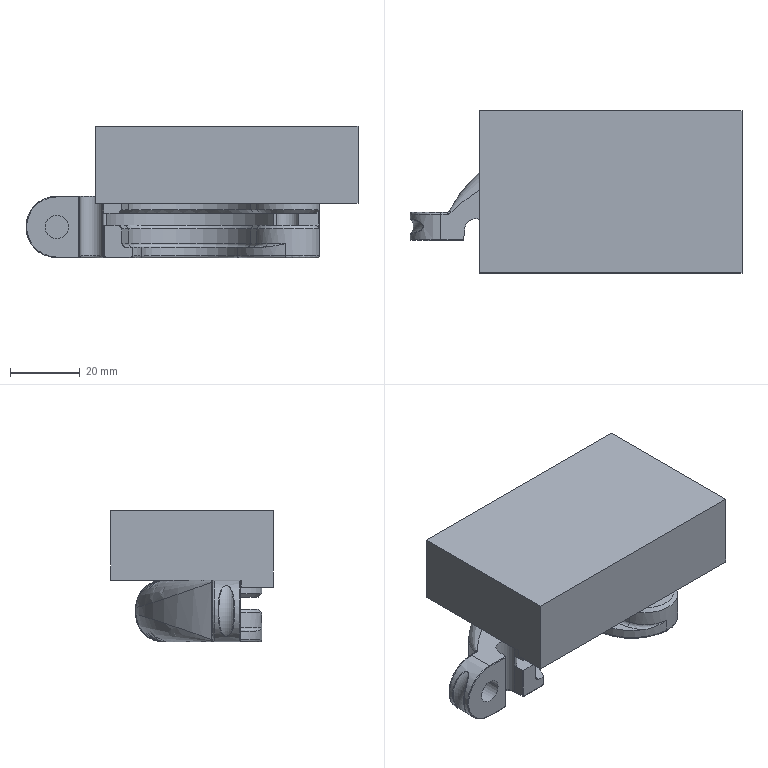NC program | NX | posted with a generic post | part box 94.951 x 46.35 x 37.6 mm
Lines 1 to 1739 of 15115, first 1433 of 1715 lines:
N10 G17 G21 G94 G90
(FACE_MILLING , TOOL : D63面刀)
N12 T01 M6
N14 G54
N16 G17 G0 G90 X104.291 Y-3.752 S4500 M3
N18 G43 Z20. H1
N20 Z3.
N22 G94 G1 Z0. F900.
N24 X72.643
N26 X-64.675 F1500.
N28 X-96.175
N30 Z3.
N32 G0 Z20.
N34 M5
(ADAPTIVE_MILLING , TOOL : D8开粗)
N36 T19 M6
N38 G54
N40 G17 G0 G90 X-51.02 Y-4.719 S6500 M3
N42 G43 Z20. H19
N44 Z-17.
N46 G94 G1 Z-20. F2100.
N48 X-49.643 Y-4.596 F3500.
N50 G3 X-49.006 Y-4.179 R0.813
N52 X-48.262 Y-1.372 R7.176
N54 X-47.978 Y7.018 R88.809
N56 G1 X-47.951 Y18.882
N58 G2 X-45.584 Y22.239 R4.73
N60 X-40.599 Y23.745 R12.005
N62 X-30.984 Y24.063 R95.907
N64 G1 X-26.234 Y24.068
N66 X42.508 Y24.067
N68 G2 X45.905 Y21.99 R4.502
N70 X47.594 Y17.053 R10.976
N72 X47.954 Y8.941 R70.776
N74 G1 X47.967 Y2.441
N76 X47.966 Y-18.643
N78 G2 X45.892 Y-22.039 R4.468
N80 X41.089 Y-23.684 R10.837
N82 X32.103 Y-24.059 R75.64
N84 G1 X25.978 Y-24.068
N86 X-42.494 Y-24.067
N88 G2 X-45.912 Y-22.034 R4.428
N90 X-47.595 Y-17.116 R10.874
N92 X-47.953 Y-9.129 R69.614
N94 X-47.555 Y-3.593 R27.936
N96 G3 X-46.984 Y8.023 R94.067
N98 G2 X-46.932 Y16.506 R267.577
N100 X-43.634 Y21.111 R6.219
N102 X-37.776 Y22.742 R14.951
N104 X-27.66 Y23.063 R109.609
N106 G1 X-23.535 Y23.067
N108 X39.857 Y23.066
N110 G2 X44.856 Y19.967 R6.087
N112 X46.593 Y14.273 R13.924
N114 X46.959 Y4.66 R91.618
N116 G1 X46.967 Y-2.215
N118 X46.944 Y-16.393
N120 G2 X43.82 Y-21.002 R6.125
N122 X38.236 Y-22.689 R13.96
N124 X28.476 Y-23.057 R91.812
N126 G1 X23.476 Y-23.067
N128 X-39.918 Y-23.065
N130 G2 X-44.82 Y-20.054 R6.012
N132 X-46.553 Y-14.619 R13.397
N134 X-46.497 Y-3.336 R45.895
N136 G3 X-45.978 Y10.393 R148.883
N138 G2 X-45.891 Y14.755 R46.886
N140 X-42.059 Y20.004 R7.121
N142 X-35.83 Y21.713 R16.455
N144 X-25.965 Y22.059 R104.665
N146 G1 X-19.09 Y22.067
N148 X0.976
N150 X2.332 Y22.205
N152 G2 X8.926 Y22.127 R73.557
N154 G1 X15.608 Y22.068
N156 X37.558 Y22.065
N158 G2 X43.868 Y18.207 R7.099
N160 X45.592 Y12.1 R16.115
N162 X45.96 Y1.611 R105.759
N164 G1 X45.967 Y-6.863
N166 X46.121 Y-7.731
N168 G2 X45.929 Y-14.694 R100.465
N170 X42.014 Y-20.037 R7.181
N172 X36.996 Y-21.568 R15.133
N174 G1 X36.466 Y-21.769
N176 X34.201 Y-22.204
N178 G2 X28.896 Y-22.118 R65.764
N180 G1 X22.206 Y-22.068
N182 X-37.544 Y-22.067
N184 G2 X-43.799 Y-18.344 R7.037
N186 X-45.264 Y-14.372 R14.785
N188 X-46.031 Y-12.836 R5.048
N190 X-46.028 Y-8.948 R12.446
N192 G3 X-45.885 Y-7.084 R20.16
N194 G2 X-46.174 Y-4.608 R6.372
N196 X-45.719 Y-2.074 R11.118
N198 G3 X-45.051 Y6.078 R50.118
N200 G2 X-44.918 Y12.773 R198.768
N202 X-40.696 Y18.891 R7.78
N204 X-34.228 Y20.679 R17.366
N206 X-23.115 Y21.061 R112.747
N208 G1 X-18.99 Y21.067
N210 X-5.419 Y21.068
N212 X-1.618 Y21.803
N214 X2.332 Y22.205
N216 X6.303 Y22.25
N218 X10.261 Y21.94
N220 G3 X19.395 Y21.101 R42.809
N222 G1 X35.932 Y21.055
N224 G2 X42.861 Y16.652 R7.812
N226 X44.595 Y10.17 R17.88
N228 X44.96 Y-0.694 R114.167
N230 G1 X44.989 Y-3.46
N232 X45.717 Y-5.46
N234 X45.98 Y-6.937
N236 G3 X47.568 Y-6.813 R0.8
N238 G1 X47.661 Y-5.251 Z-19.9
N240 X47.74 Y-3.888
N242 X47.702 Y-0.81
N244 X47.617 Y2.267
N246 X47.499 Y4.315
N248 X47.338 Y6.36
N250 X47.052 Y9.524
N252 X46.747 Y12.687
N254 G3 X45.741 Y16.134 R13.079
N256 X44.088 Y19.29 R24.994
N258 X37.545 Y23.22 R8.856
N260 X33.163 Y23.495 R58.704
N262 G1 X15.727 Y23.898
N264 X15.524 Y23.849
N266 X14.073 Y23.289
N268 X13.077 Y22.895 Z-19.969
N270 G3 X12.75 Y22.537 Z-20. R0.846
N272 X13.342 Y21.413 R0.8
N274 G2 X16.779 Y20.595 R32.188
N276 G3 X23.653 Y20.109 R41.473
N278 G1 X34.557 Y20.036
N280 G2 X41.838 Y15.239 R8.359
N282 X43.576 Y8.62 R18.862
N284 X43.964 Y-1.334 R112.841
N286 G1 X44.021 Y-1.556
N288 G2 X45.014 Y-3.527 R30.259
N290 G3 X46.304 Y-3.845 R0.8
N292 X46.574 Y-3.166 Z-19.952 R0.899
N294 G1 X46.635 Y-2.357 Z-19.9
N296 X46.774 Y-0.478
N298 X46.776 Y1.281
N300 X46.73 Y3.039
N302 X46.635 Y4.206
N304 X46.497 Y5.37
N306 X45.704 Y10.852
N308 G3 X44.528 Y15.045 R20.143
N310 X43.203 Y17.473 R13.919
N312 G1 X42.516 Y18.481
N314 X41.794 Y19.464
N316 G3 X41.087 Y20.126 R3.656
N318 X36.954 Y22.042 R11.259
N320 G1 X36.341 Y22.149
N322 X35.722 Y22.22
N324 X32.067 Y22.476
N326 X28.41 Y22.683
N328 X19.055 Y23.131
N330 X18.882 Y23.116
N332 X18.714 Y23.072
N334 X17.29 Y22.49
N336 X16.816 Y22.298 Z-19.933
N338 X16.349 Y22.093 Z-19.965
N340 G3 X16.016 Y21.677 Z-20. R0.837
N342 X16.565 Y20.641 R0.8
N344 G2 X19.636 Y19.719 R46.577
N346 G3 X25.689 Y19.144 R31.586
N348 G2 X33.243 Y19.021 R667.849
N350 X40.794 Y13.949 R8.781
N352 X42.57 Y7.089 R19.793
N354 X42.94 Y0.558 R126.133
N356 G3 X44.028 Y-1.57 R111.415
N358 X45.191 Y-1.858 R0.8
N360 X45.547 Y-1.135 Z-19.947 R0.881
N362 G1 X45.621 Y-0.413 Z-19.9
N364 X45.796 Y1.382
N366 X45.252 Y5.256
N368 X44.683 Y9.127
N370 G3 X43.427 Y13.856 R27.88
N372 G1 X42.817 Y15.509
N374 G3 X41.412 Y17.59 R6.625
N376 X38.104 Y20.149 R16.811
N378 X35.162 Y21.088 R8.045
N380 G1 X32.008 Y21.444
N382 X28.848 Y21.745
N384 X21.628 Y22.348
N386 X21.431 Y22.337
N388 X21.24 Y22.283
N390 X19.885 Y21.688
N392 X18.991 Y21.287 Z-19.963
N394 G3 X18.647 Y20.83 Z-20. R0.83
N396 X19.139 Y19.858 R0.801
N398 X22.763 Y18.649 R25.814
N400 X29.299 Y18.13 R40.933
N402 G2 X34.012 Y17.673 R18.904
N404 X39.845 Y12.527 R9.247
N406 X41.589 Y5.394 R21.313
N408 G1 X41.851 Y2.231
N410 G3 X43.044 Y0.313 R15.776
N412 X44.116 Y0.055 R0.801
N414 X44.528 Y0.799 Z-19.943 R0.875
N416 G1 X44.61 Y1.469 Z-19.9
N418 X44.726 Y2.352
N420 X44.818 Y3.237
N422 G3 X42.965 Y11.077 R64.156
N424 X41.261 Y14.968 R19.576
N426 G1 X40.36 Y16.513
N428 G3 X38.875 Y17.974 R5.483
N430 X33.742 Y20.116 R13.869
N432 G1 X32.664 Y20.317
N434 X31.579 Y20.481
N436 X23.982 Y21.446
N438 X23.82 Y21.424
N440 X23.663 Y21.376
N442 X22.341 Y20.784
N444 X21.449 Y20.376 Z-19.963
N446 G3 X21.109 Y19.918 Z-20. R0.83
N448 X21.602 Y18.95 R0.801
N450 G1 X23.779 Y18.005
N452 G3 X28.447 Y17.268 R19.998
N454 G2 X33.008 Y16.627 R19.382
N456 X38.887 Y11.172 R9.701
N458 X40.548 Y4.469 R22.433
N460 G3 X40.836 Y3.73 R1.258
N462 G1 X41.921 Y2.05
N464 G3 X43.335 Y2.185 R0.8
N466 X43.335 Y2.857 Z-19.956 R1.091
N468 G1 X43.162 Y3.72 Z-19.9
N470 X42.836 Y5.372
N472 X42.831 Y5.98
N474 X42.785 Y6.587
N476 G3 X41.688 Y10.669 R25.729
N478 X40.431 Y13.306 R16.27
N480 G1 X39.455 Y14.928
N482 G3 X37.035 Y17.302 R8.254
N484 X33.086 Y19.162 R13.784
N486 X31.176 Y19.51 R11.526
N488 G1 X26.234 Y19.969
N490 X24.471 Y19.81
N492 X23.408 Y19.703 Z-19.968
N494 G3 X22.994 Y19.445 Z-20. R0.845
N496 X23.259 Y18.205 R0.8
N498 X26.334 Y16.884 R18.397
N500 X30.452 Y16.102 R99.604
N502 G2 X37.924 Y9.88 R10.25
N504 X39.185 Y5.864 R27.369
N506 G1 X40.782 Y3.799
N508 G3 X42.064 Y3.832 R0.8
N510 X42.172 Y4.584 Z-19.95 R0.9
N512 G1 X42.039 Y5.352 Z-19.9
N514 X41.728 Y7.106
N516 X40.782 Y9.234
N518 X39.816 Y11.353
N520 G3 X36.767 Y15.518 R13.967
N522 X33.532 Y17.631 R12.909
N524 X31.698 Y18.233 R10.561
N526 G1 X28.338 Y18.996
N528 X28.08 Y19.012
N530 X26.479 Y18.849
N532 X25.428 Y18.731 Z-19.968
N534 G3 X25.011 Y18.46 Z-20. R0.843
N536 X25.289 Y17.236 R0.8
N538 G1 X27.065 Y16.272
N540 X30.763 Y14.957
N542 G2 X37.032 Y8.501 R11.31
N544 G1 X37.242 Y8.072
N546 G2 X39.25 Y5.75 R19.09
N548 G3 X40.548 Y5.805 R0.8
N550 X40.638 Y6.536 Z-19.951 R0.896
N552 G1 X40.488 Y7.327 Z-19.9
N554 X40.39 Y7.864
N556 X40.274 Y8.398
N558 X40.179 Y8.574
N560 X40.047 Y8.725
N562 X29.323 Y18.01
N564 G3 X28.686 Y18.197 R0.808
N566 G1 X27.817 Y18.073
N568 X27.316 Y18.003 Z-19.932
N570 X26.817 Y17.918 Z-19.965
N572 G3 X26.39 Y17.586 Z-20. R0.836
N574 X26.656 Y16.47 R0.8
N576 G2 X31.937 Y13.115 R52.707
N578 X33.4 Y11.755 R22.501
N580 X37.246 Y8.068 R34.365
N582 G3 X38.5 Y9.053 R0.801
N584 G1 X37.718 Y10.408 Z-19.9
N586 X37.331 Y11.058
N588 X37.246 Y11.149
N590 X32.159 Y15.761
N592 X31.989 Y15.876
N594 X31.797 Y15.949
N596 X30.891 Y16.153
N598 X29.712 Y16.409 Z-19.977
N600 X29.534 Y16.398 Z-19.989
N602 X29.361 Y16.355 Z-20.
N604 G3 X29.184 Y14.964 R0.8
N606 G1 X32.473 Y12.57
N608 X33.412 Y11.745
N610 G3 X34.209 Y11.592 R0.803
N612 G1 X34.462 Y11.739 Z-19.981
N614 X34.685 Y11.928 Z-19.963
N616 X35.434 Y12.558 Z-19.9
N618 X35.651 Y12.742
N620 X35.894 Y12.893
N622 G2 X36.812 Y12.656 R0.801
N624 G1 X40.201 Y8.483
N626 G2 X43.948 Y3.357 R76.172
N628 X45.937 Y-0.004 R46.197
N630 G1 X47.032 Y-2.073
N632 G2 X48.199 Y-5.501 R14.427
N634 G1 X48.618 Y-7.549
N636 G2 X48.259 Y-8.387 R0.802
N638 G1 X48.104 Y-8.484
N640 X46.778 Y-9.316 Z-20.
N642 X46.521 Y-9.475
N644 G3 X46.128 Y-10.038 R0.908
N646 G2 X45.654 Y-12.547 R19.534
N648 X43.824 Y-16.49 R11.526
N650 G1 X42.358 Y-18.271
N652 X40.607 Y-19.772
N654 X38.623 Y-20.95
N656 X36.987 Y-21.571
N658 G3 X36.606 Y-22.764 R0.8
N660 X37.292 Y-23.133 Z-19.948 R0.892
N662 G1 X38.039 Y-23.255 Z-19.9
N664 X38.795 Y-23.384
N666 X39.555 Y-23.491
N668 G3 X40.036 Y-23.331 R0.825
N670 G1 X42.47 Y-21.491
N672 G3 X45.378 Y-18.415 R16.117
N674 G1 X47.414 Y-15.596
N676 G3 X47.556 Y-15.005 R0.812
N678 G1 X47.348 Y-13.658
N680 X47.172 Y-12.579 Z-19.97
N682 G3 X46.912 Y-12.195 Z-20. R0.852
N684 X45.654 Y-12.547 R0.8
N686 G1 X44.962 Y-14.484
N688 X43.824 Y-16.49
N690 X42.358 Y-18.271
N692 X40.607 Y-19.772
N694 X38.623 Y-20.95
N696 X36.466 Y-21.769
N698 X34.201 Y-22.204
N700 X31.895 Y-22.242
N702 X29.155 Y-21.851
N704 G3 X24.557 Y-21.196 R17.279
N706 X14.706 Y-21.068 R300.396
N708 G1 X-35.494 Y-21.066
N710 G2 X-42.791 Y-16.805 R7.835
N712 G3 X-43.475 Y-15.763 R3.342
N714 G2 X-45.347 Y-14.231 R4.167
N716 G3 X-46.728 Y-15.009 R0.8
N718 G1 X-46.029 Y-16.408 Z-19.9
N720 X-45.347 Y-17.751
N722 X-44.862 Y-18.482
N724 X-44.341 Y-19.189
N726 X-43.95 Y-19.622
N728 X-43.532 Y-20.029
N730 X-42.119 Y-21.273
N732 G3 X-36.704 Y-23.29 R8.961
N734 G1 X-34.755 Y-23.394
N736 X-32.804 Y-23.447
N738 X26.052 Y-24.123
N740 X26.258 Y-24.069
N742 X27.697 Y-23.481
N744 X28.169 Y-23.29 Z-19.933
N746 X28.634 Y-23.085 Z-19.965
N748 G3 X28.967 Y-22.664 Z-20. R0.836
N750 X28.435 Y-21.64 R0.8
N752 X25.125 Y-20.647 R152.961
N754 X18.279 Y-20.117 R39.289
N756 G1 X10.831 Y-20.068
N758 X-33.619 Y-20.066
N760 G2 X-38.961 Y-18.63 R9.039
N762 X-41.575 Y-16.272 R25.088
N764 G1 X-41.929 Y-16.103
N766 G2 X-43.601 Y-15.689 R4.008
N768 G3 X-44.704 Y-16.364 R0.8
N770 X-44.429 Y-17.052 Z-19.951 R0.894
N772 G1 X-43.917 Y-17.666 Z-19.9
N774 X-42.781 Y-19.019
N776 X-41.518 Y-19.872
N778 X-40.243 Y-20.707
N780 G3 X-35.676 Y-22.237 R11.641
N782 X-32.268 Y-22.421 R35.503
N784 G1 X23.411 Y-22.775
N786 X25.17 Y-22.624
N788 X26.241 Y-22.522 Z-19.969
N790 G3 X26.653 Y-22.274 Z-20. R0.847
N792 X26.386 Y-21.018 R0.8
N794 X23.294 Y-19.769 R16.508
N796 X16.751 Y-19.147 R34.278
N798 X6.832 Y-19.068 R613.153
N800 G1 X-31.618 Y-19.067
N802 G2 X-36.626 Y-18.205 R11.616
N804 X-39.691 Y-16.358 R25.242
N806 G3 X-40.254 Y-16.125 R2.099
N808 G2 X-42.01 Y-16.093 R37.287
N810 G3 X-42.892 Y-17.069 R0.8
N812 X-42.421 Y-17.638 Z-19.951 R0.895
N814 G1 X-41.746 Y-18.071 Z-19.9
N816 X-41.248 Y-18.393
N818 X-40.74 Y-18.7
N820 X-40.47 Y-18.76
N822 X21.829 Y-21.672
N824 X23.097 Y-21.665
N826 X23.678 Y-21.663 Z-19.937
N828 X24.259 Y-21.646 Z-19.974
N830 X24.449 Y-21.584 Z-19.987
N832 X24.622 Y-21.482 Z-20.
N834 G3 X24.455 Y-20.131 R0.8
N836 G2 X23.154 Y-19.4 R10.946
N838 G3 X18.77 Y-18.391 R13.255
N840 X8.823 Y-18.077 R119.783
N842 G1 X-29.244 Y-18.069
N844 G2 X-34.207 Y-17.621 R18.247
N846 X-37.772 Y-16.167 R22.758
N848 G1 X-37.959 Y-16.125
N850 X-40.334
N852 G3 X-40.379 Y-17.884 R0.88
N854 G1 X-38.122 Y-17.999
N856 X-36.559 Y-18.08 Z-19.9
N858 X22.182 Y-21.092
N860 X22.962 Y-21.122 Z-19.95
N862 G3 X23.611 Y-20.73 Z-20. R0.895
N864 X23.355 Y-19.507 R0.88
N866 X20.583 Y-18.043 R9.835
N868 X14.436 Y-17.225 R26.833
N870 X2.332 Y-17.069 R314.868
N872 G1 X-34.442 Y-17.047
N874 X-35.922 Y-16.185
N876 X-36.168 Y-16.125
N878 X-38.043
N880 G3 X-38.078 Y-17.884 R0.88
N882 G1 X-34.699 Y-18.018
N884 X-33.136 Y-18.08 Z-19.9
N886 X20.83 Y-20.217
N888 X21.608 Y-20.238 Z-19.95
N890 G3 X22.254 Y-19.836 Z-20. R0.895
N892 X21.991 Y-18.624 R0.88
N894 G2 X20.98 Y-17.855 R23.145
N896 G3 X16.757 Y-16.576 R11.091
N898 X7.181 Y-16.094 R80.358
N900 G1 X1.706 Y-16.069
N902 X-11.094
N904 X-11.564 Y-16.125
N906 G2 X-26.403 Y-16.073 R924.171
N908 G1 X-26.834 Y-16.125
N910 X-36.209
N912 G3 X-36.505 Y-17.668 R0.8
N914 G1 X-34.995 Y-18.075 Z-19.9
N916 X-34.135 Y-18.296
N918 X-21.696 Y-18.303
N920 X-21.484 Y-18.274
N922 X-20.52 Y-18.009
N924 X-19.257 Y-17.65 Z-19.984
N926 X-19.048 Y-17.513 Z-20.
N928 G3 X-19.518 Y-16.125 R0.8
N930 G2 X-21.575 Y-15.691 R5.213
N932 G3 X-24.205 Y-15.318 R11.691
N934 X-24.793 Y-15.623 R1.742
N936 G2 X-26.403 Y-16.073 R4.48
N938 G3 X-26.344 Y-17.825 R0.88
N940 G1 X-24.785 Y-17.705 Z-19.9
N942 X-22.31 Y-17.501
N944 X-21.876 Y-17.47 Z-19.928
N946 X-21.446 Y-17.407 Z-19.956
N948 G3 X-20.924 Y-16.978 Z-20. R0.886
N950 X-21.408 Y-15.739 R0.88
N952 G2 X-22.367 Y-15.202 R9.846
N954 G3 X-23.766 Y-14.952 R1.975
N956 G1 X-24.539 Y-15.449
N958 G3 X-24.812 Y-16.596 R0.881
N960 X-23.863 Y-17.048 Z-19.929 R0.934
N962 G1 X-23.418 Y-17.034 Z-19.9
N964 X-23.106 Y-17.023
N966 X-22.339 Y-16.988 Z-19.949
N968 G3 X-21.72 Y-16.531 Z-20. R0.895
N970 X-22.007 Y-15.393 R0.881
N972 X-23.018 Y-14.748 R6.658
N974 X-24.024 Y-15.095 R1.114
N976 X-23.127 Y-16.604 R0.88
N978 G1 X-22.644 Y-16.346
N980 G3 X-22.5 Y-15.06 R0.88
N982 X-23.87 Y-14.967 R0.874
N984 X-24.064 Y-15.485 R0.819
N986 G1 X-24.065 Y-15.871
N988 X-24.069 Y-17.436 Z-19.9
N990 G2 X-24.782 Y-18.367 R0.834
N992 G1 X-26.53 Y-18.563
N994 X-28.282 Y-18.714
N996 X-29.453 Y-18.753
N998 X-30.624 Y-18.751
N1000 X-42.659 Y-18.456
N1002 G2 X-47.681 Y-15.035 R5.577
N1004 G1 X-48.65 Y-12.703
N1006 G2 X-48.158 Y-11.623 R0.832
N1008 G1 X-46.768 Y-10.903 Z-20.
N1010 G3 X-46.236 Y-10.454 R1.036
N1012 X-45.987 Y-9.024 R10.911
N1014 X-45.577 Y-7.92 R3.207
N1016 X-45.945 Y-6.889 R3.239
N1018 G2 X-46.174 Y-4.608 R6.402
N1020 G1 X-46.048 Y-3.343
N1022 G2 X-45.129 Y-1.225 R23.425
N1024 G3 X-44.22 Y4.097 R19.795
N1026 X-43.954 Y10.936 R538.277
N1028 G2 X-39.17 Y17.933 R8.368
N1030 X-32.558 Y19.675 R18.833
N1032 X-21.819 Y20.058 R112.509
N1034 G1 X-8.882 Y20.078
N1036 X-5.394 Y21.073
N1038 G3 X-5.17 Y22.565 R0.8
N1040 X-5.726 Y22.671 Z-19.964 R1.279
N1042 G1 X-6.718 Y22.73 Z-19.9
N1044 X-8.443 Y22.833
N1046 X-22.622
N1048 G3 X-31.385 Y22.252 R66.484
N1050 G1 X-33.242 Y22.008
N1052 X-35.093 Y21.723
N1054 G3 X-39.193 Y20.556 R21.136
N1056 X-42.298 Y18.863 R17.245
N1058 X-45.501 Y14.532 R9.105
N1060 X-46.164 Y11.699 R12.855
N1062 G1 X-46.42 Y9.764
N1064 X-46.642 Y7.824
N1066 X-47.352 Y0.799
N1068 X-47.134 Y-0.924
N1070 X-46.999 Y-1.896 Z-19.963
N1072 G3 X-46.66 Y-2.354 Z-20. R0.83
N1074 X-45.588 Y-2.158 R0.801
N1076 X-43.64 Y2.224 R8.412
N1078 X-43.042 Y9.021 R55.93
N1080 G2 X-37.661 Y17.002 R9.017
N1082 X-30.774 Y18.695 R20.684
N1084 X-18.659 Y19.062 R136.64
N1086 G1 X-11.643 Y19.075
N1088 G2 X-8.851 Y20.087 R56.002
N1090 G3 X-8.598 Y21.499 R0.8
N1092 X-9.24 Y21.669 Z-19.957 R1.099
N1094 G1 X-10.126 Y21.729 Z-19.9
N1096 X-11.9 Y21.847
N1098 X-20.701
N1100 G3 X-30.431 Y21.156 R68.93
N1102 G1 X-33.977 Y20.638
N1104 G3 X-38.469 Y19.26 R20.042
N1106 X-40.74 Y17.861 R12.305
N1108 X-43.034 Y15.917 R26.005
N1110 X-44.586 Y13.191 R6.411
N1112 X-45.647 Y8.034 R54.798
N1114 G1 X-46.597 Y1.816
N1116 X-46.58 Y1.626
N1118 X-46.282 Y0.2
N1120 X-46.062 Y-0.799 Z-19.965
N1122 G3 X-45.715 Y-1.201 Z-20. R0.837
N1124 X-44.828 Y-1.138 R0.802
N1126 X-43.333 Y1.006 R4.387
N1128 X-42.288 Y6.422 R20.895
N1130 G2 X-41.317 Y11.173 R14.886
N1132 X-35.891 Y16.21 R9.905
N1134 X-28.46 Y17.768 R24.307
N1136 X-16.216 Y18.06 R169.565
N1138 G3 X-13.9 Y18.097 R32.081
N1140 G2 X-11.401 Y19.144 R25.984
N1142 G3 X-11.116 Y20.446 R0.8
N1144 X-11.78 Y20.699 Z-19.953 R0.909
N1146 G1 X-12.612 Y20.764 Z-19.9
N1148 X-14.45 Y20.904
N1150 X-20.106 Y20.892
N1152 G3 X-27.613 Y20.323 R66.627
N1154 G1 X-30.117 Y19.993
N1156 X-32.618 Y19.644
N1158 G3 X-38.624 Y17.497 R17.75
N1160 G1 X-39.577 Y16.903
N1162 X-40.5 Y16.263
N1164 G3 X-42.542 Y13.944 R7.544
N1166 G1 X-43.061 Y13.008
N1168 X-43.539 Y12.05
N1170 G3 X-44.412 Y9.087 R11.849
N1172 G1 X-45.444 Y2.48
N1174 X-45.695 Y0.687
N1176 X-45.822 Y-0.282 Z-19.963
N1178 G3 X-45.612 Y-0.816 Z-20. R0.83
N1180 X-44.531 Y-0.908 R0.801
N1182 X-42.34 Y2.064 R5.447
N1184 X-41.282 Y6.99 R29.351
N1186 G2 X-34.938 Y15.086 R10.225
N1188 X-27.65 Y16.715 R23.77
N1190 X-16.064 Y17.067 R152.795
N1192 G1 X-15.834 Y17.121
N1194 X-13.706 Y18.176
N1196 G3 X-13.419 Y19.369 R0.8
N1198 X-14.137 Y19.703 Z-19.947 R0.886
N1200 G1 X-14.876 Y19.77 Z-19.9
N1202 X-16.755 Y19.936
N1204 X-18.791 Y19.939
N1206 X-20.827 Y19.9
N1208 G3 X-24.068 Y19.613 R38.508
N1210 G1 X-27.541 Y19.156
N1212 X-31.012 Y18.678
N1214 G3 X-37.765 Y16.422 R21.755
N1216 G1 X-38.482 Y16.043
N1218 X-39.177 Y15.625
N1220 G3 X-40.444 Y14.389 R5.895
N1222 X-41.789 Y12.351 R18.343
N1224 X-43.311 Y8.796 R13.848
N1226 G1 X-44.047 Y5.925
N1228 X-44.734 Y3.042
N1230 X-44.809 Y2.18
N1232 X-44.864 Y1.316
N1234 X-44.901 Y0.809 Z-19.933
N1236 X-44.922 Y0.3 Z-19.965
N1238 G3 X-44.692 Y-0.184 Z-20. R0.837
N1240 X-43.823 Y-0.359 R0.802
N1242 X-42.068 Y1.358 R3.547
N1244 X-40.861 Y4.681 R13.407
N1246 G2 X-39.305 Y9.281 R18.37
N1248 X-33.105 Y14.347 R11.283
N1250 X-25.14 Y15.806 R28.758
N1252 X-17.772 Y16.071 R356.89
N1254 G3 X-16.59 Y16.746 R5.631
N1256 G1 X-15.806 Y17.135
N1258 G3 X-15.515 Y18.323 R0.8
N1260 X-16.233 Y18.662 Z-19.947 R0.885
N1262 G1 X-16.969 Y18.731 Z-19.9
N1264 X-18.778 Y18.899
N1266 G3 X-28.894 Y17.818 R301.348
N1268 X-33.868 Y16.673 R31.685
N1270 X-40.987 Y11.139 R13.365
N1272 X-41.886 Y9.398 R12.632
N1274 G1 X-44.503 Y3.137
N1276 X-44.563 Y2.873
N1278 X-44.643 Y1.436
N1280 X-44.691 Y0.391 Z-19.967
N1282 G3 X-44.478 Y-0.072 Z-20. R0.841
N1284 X-43.591 Y-0.264 R0.802
N1286 X-41.251 Y1.759 R4.029
N1288 X-39.639 Y5.733 R24.711
N1290 G2 X-31.909 Y13.372 R12.031
N1292 X-23.684 Y14.815 R30.538
N1294 G1 X-19.447 Y15.034
N1296 G3 X-17.584 Y16.136 R18.448
N1298 X-17.318 Y17.231 R0.801
N1300 X-18.063 Y17.63 Z-19.944 R0.877
N1302 G1 X-18.74 Y17.707 Z-19.9
N1304 X-20.531 Y17.904
N1306 X-24.132 Y17.4
N1308 X-27.729 Y16.872
N1310 G3 X-33.209 Y15.453 R32.406
N1312 X-37.95 Y12.649 R15.314
N1314 X-40.952 Y8.835 R13.486
N1316 G1 X-43.809 Y3.422
N1318 X-43.87 Y3.256
N1320 X-43.9 Y3.083
N1322 X-43.96 Y1.727
N1324 X-43.996 Y0.67 Z-19.968
N1326 G3 X-43.788 Y0.218 Z-20. R0.843
N1328 X-42.898 Y0.021 R0.802
N1330 X-40.531 Y1.926 R4.064
N1332 X-38.654 Y5.606 R39.509
N1334 G2 X-30.342 Y12.541 R13.223
N1336 X-21.843 Y13.853 R35.407
N1338 G3 X-20.821 Y14.039 R2.691
N1340 G2 X-19.229 Y15.127 R16.242
N1342 G3 X-18.96 Y16.219 R0.801
N1344 X-19.703 Y16.621 Z-19.944 R0.877
N1346 G1 X-20.379 Y16.701 Z-19.9
N1348 X-21.267 Y16.81
N1350 X-22.156 Y16.901
N1352 G3 X-27.535 Y15.799 R83.69
N1354 G1 X-29.704 Y15.208
N1356 X-31.858 Y14.566
N1358 G3 X-36.806 Y11.71 R14.901
N1360 X-39.39 Y8.836 R13.056
N1362 X-42.686 Y3.569 R94.911
N1364 G1 X-43.216 Y2.013
N1366 X-43.381 Y1.53 Z-19.933
N1368 X-43.531 Y1.043 Z-19.965
N1370 G3 X-43.434 Y0.519 Z-20. R0.837
N1372 X-42.646 Y0.124 R0.802
N1374 X-40.264 Y1.43 R3.352
N1376 X-38.051 Y4.756 R23.95
N1378 G2 X-28.742 Y11.713 R14.815
N1380 X-22.691 Y12.753 R43.91
N1382 G1 X-22.401 Y12.863
N1384 X-20.796 Y14.058
N1386 G3 X-20.855 Y15.381 R0.8
N1388 X-21.568 Y15.458 Z-19.953 R0.905
N1390 G1 X-22.38 Y15.307 Z-19.9
N1392 X-24.197 Y14.969
N1394 X-27.739 Y14.426
N1396 G3 X-34.867 Y11.607 R19.223
N1398 X-37.488 Y9.286 R12.98
N1400 X-42.206 Y3.624 R156.975
N1402 G1 X-42.289 Y3.447
N1404 X-42.721 Y2.107
N1406 X-43.035 Y1.1 Z-19.968
N1408 G3 X-42.953 Y0.606 Z-20. R0.842
N1410 X-42.15 Y0.183 R0.802
N1412 X-39.509 Y1.509 R3.763
N1414 X-36.733 Y4.975 R47.099
N1416 G2 X-27.252 Y10.849 R16.514
N1418 G1 X-24.074 Y11.528
N1420 G3 X-23.159 Y12.298 R8.028
N1422 G1 X-22.357 Y12.896
N1424 G3 X-22.533 Y14.278 R0.8
N1426 X-23.174 Y14.277 Z-19.958 R0.935
N1428 G1 X-24.057 Y14.059 Z-19.9
N1430 X-25.165 Y13.78
N1432 X-25.333 Y13.693
N1434 X-40.811 Y3.171
N1436 X-41.654 Y2.226
N1438 X-42.294 Y1.488 Z-19.963
N1440 G3 X-42.414 Y0.927 Z-20. R0.83
N1442 X-41.529 Y0.257 R0.801
N1444 X-38.996 Y1.28 R3.67
N1446 X-35.741 Y4.614 R47.051
N1448 G2 X-26.938 Y9.707 R18.274
N1450 G3 X-25.568 Y10.144 R6.881
N1452 G1 X-23.891 Y11.644
N1454 G3 X-24.895 Y13.074 R0.88
N1456 G1 X-26.195 Y12.203 Z-19.9
N1458 X-40.969 Y2.242
N1460 X-41.602 Y1.803 Z-19.949
N1462 G3 X-41.884 Y1.09 Z-20. R0.895
N1464 X-41.007 Y0.275 R0.881
N1466 X-38.262 Y1.187 R4.053
N1468 X-34.64 Y4.294 R56.95
N1470 G2 X-27.386 Y8.38 R21.573
N1472 G1 X-27.176 Y8.519
N1474 G2 X-25.56 Y10.151 R18.369
N1476 G3 X-26.383 Y11.654 R0.88
N1478 G1 X-26.648 Y11.531 Z-19.981
N1480 X-26.889 Y11.366 Z-19.963
N1482 X-27.699 Y10.817 Z-19.9
N1484 X-40.346 Y2.242
N1486 X-40.979 Y1.801 Z-19.949
N1488 G3 X-41.259 Y1.088 Z-20. R0.895
N1490 X-40.382 Y0.275 R0.881
N1492 X-37.272 Y1.184 R4.84
N1494 X-33.062 Y4.234 R144.456
N1496 G2 X-29.037 Y6.521 R32.837
N1498 G1 X-27.122 Y8.576
N1500 G3 X-27.682 Y10.053 R0.88
N1502 X-28.38 Y9.823 Z-19.952 R0.989
N1504 G1 X-29.052 Y9.369 Z-19.9
N1506 X-39.596 Y2.241
N1508 X-40.228 Y1.802 Z-19.949
N1510 G3 X-40.509 Y1.087 Z-20. R0.895
N1512 X-39.632 Y0.275 R0.881
N1514 X-36.087 Y1.19 R5.83
N1516 G2 X-30.528 Y4.575 R724.732
N1518 G1 X-28.889 Y6.671
N1520 G3 X-29.286 Y8.04 R0.88
N1522 X-30.196 Y7.86 Z-19.938 R0.95
N1524 G1 X-30.69 Y7.53 Z-19.9
N1526 X-38.588 Y2.244
N1528 X-39.225 Y1.805 Z-19.95
N1530 G3 X-39.51 Y1.096 Z-20. R0.895
N1532 X-38.632 Y0.275 R0.881
N1534 X-34.76 Y1.156 R7.018
N1536 X-31.934 Y2.66 R196.592
N1538 X-31.267 Y3.615 R4.897
N1540 G1 X-30.5 Y4.602
N1542 G3 X-30.844 Y5.95 R0.88
N1544 X-31.784 Y5.811 Z-19.936 R0.942
N1546 G1 X-32.263 Y5.508 Z-19.9
N1548 X-37.433 Y2.243
N1550 X-38.082 Y1.821 Z-19.95
N1552 G3 X-38.386 Y1.12 Z-20. R0.895
N1554 X-37.507 Y0.275 R0.881
N1556 X-32.779 Y1.348 R8.46
N1558 X-31.757 Y2.855 R10.148
N1560 X-32.039 Y4.083 R0.88
N1562 X-33.072 Y4.015 Z-19.93 R0.941
N1564 G1 X-33.476 Y3.781 Z-19.9
N1566 X-36.138 Y2.24
N1568 X-36.806 Y1.843 Z-19.95
N1570 G3 X-37.137 Y1.157 Z-20. R0.895
N1572 X-36.257 Y0.275 R0.88
N1574 X-33.726 Y0.403 R11.088
N1576 X-33.101 Y0.765 R1.212
N1578 G1 X-32.627 Y1.501
N1580 G3 X-32.971 Y2.763 R0.88
N1582 X-33.967 Y2.637 Z-19.932 R0.935
N1584 G1 X-34.389 Y2.363 Z-19.9
N1586 X-34.575 Y2.242
N1588 X-35.216 Y1.813 Z-19.949
N1590 G3 X-35.51 Y1.106 Z-20. R0.895
N1592 X-34.632 Y0.275 R0.881
N1594 X-33.474 Y0.38 R2.698
N1596 X-33.094 Y0.776 R1.58
N1598 X-33.058 Y1.579 R0.803
N1600 X-33.478 Y1.988 Z-19.962 R1.221
N1602 G1 X-34.264 Y2.559 Z-19.9
N1604 X-35.13 Y3.178
N1606 G3 X-35.583 Y3.265 R0.839
N1608 G1 X-42.392 Y2.565
N1610 G3 X-45.298 Y1.538 R6.863
N1612 X-47.908 Y-1.415 R6.345
N1614 X-48.511 Y-3.922 R10.127
N1616 G1 X-48.684 Y-5.343
N1618 X-48.809 Y-6.769
N1620 G3 X-48.731 Y-10.243 R22.385
N1622 G1 X-48.584 Y-11.723
N1624 X-48.421 Y-13.201
N1626 G3 X-46.885 Y-16.192 R5.495
N1628 G1 X-45.957 Y-17.103
N1630 G3 X-43.85 Y-18.147 R5.06
N1632 X-42.218 Y-18.389 R9.477
N1634 G1 X-40.757 Y-18.494
N1636 X-39.294 Y-18.553
N1638 X18.142 Y-19.759
N1640 X19.033 Y-19.647
N1642 X19.922 Y-19.515
N1644 X20.891 Y-19.368 Z-19.963
N1646 G3 X21.345 Y-19.021 Z-20. R0.83
N1648 X21.19 Y-17.999 R0.801
N1650 X17.21 Y-15.921 R7.528
N1652 X9.371 Y-15.166 R42.667
N1654 X-8.543 Y-15.077 R771.302
N1656 X-9.555 Y-15.64 R2.862
N1658 G2 X-11.15 Y-16.076 R4.496
N1660 G3 X-11.505 Y-17.701 R0.88
N1662 X-10.852 Y-17.836 Z-19.957 R1.208
N1664 G1 X-9.965 Y-17.864 Z-19.9
N1666 X19.093 Y-18.78
N1668 X19.868 Y-18.794 Z-19.95
N1670 G3 X20.512 Y-18.384 Z-20. R0.895
N1672 X20.344 Y-17.258 R0.881
N1674 X18.419 Y-15.771 R9.074
N1676 X13.234 Y-14.498 R15.736
N1678 X1.571 Y-14.079 R122.1
N1680 X-7.186 Y-14.119 R190.039
N1682 X-8.085 Y-14.397 R1.514
N1684 G2 X-8.899 Y-15.199 R3.409
N1686 G3 X-9.206 Y-16.299 R0.881
N1688 X-8.297 Y-16.815 Z-19.929 R0.936
N1690 G1 X-7.845 Y-16.835 Z-19.9
N1692 X18.226 Y-18.01
N1694 X19.001 Y-18.035 Z-19.95
N1696 G3 X19.65 Y-17.635 Z-20. R0.895
N1698 X19.578 Y-16.588 R0.881
N1700 X16.175 Y-14.304 R6.09
N1702 X9.522 Y-13.302 R28.826
N1704 X-5.853 Y-13.126 R213.584
N1706 X-7.451 Y-13.517 R3.267
N1708 X-7.991 Y-14.294 R3.457
N1710 G1 X-8.16 Y-14.479
N1712 G3 X-8.29 Y-15.481 R0.881
N1714 X-7.411 Y-15.959 Z-19.932 R0.937
N1716 G1 X-6.905 Y-15.985 Z-19.9
N1718 X17.55 Y-17.244
N1720 X18.342 Y-17.276 Z-19.951
N1722 G3 X18.986 Y-16.896 Z-20. R0.895
N1724 X18.928 Y-15.828 R0.881
N1726 X15.398 Y-13.388 R6.383
N1728 X8.515 Y-12.319 R29.183
N1730 X-4.834 Y-12.152 R145.566
N1732 X-6.899 Y-12.637 R4.75
N1734 X-7.668 Y-13.771 R5.332
N1736 X-7.658 Y-14.71 R0.882
N1738 X-6.817 Y-15.119 Z-19.937 R0.947
N1740 G1 X-6.233 Y-15.149 Z-19.9
N1742 X16.742 Y-16.296
N1744 X17.532 Y-16.326 Z-19.951
N1746 G3 X18.176 Y-15.943 Z-20. R0.895
N1748 X18.116 Y-14.878 R0.881
N1750 X16.763 Y-13.474 R6.765
N1752 X12.027 Y-11.829 R12.296
N1754 X2.277 Y-11.132 R68.14
N1756 X-4.587 Y-11.248 R55.68
N1758 X-6.336 Y-11.728 R4.629
N1760 X-7.103 Y-12.857 R5.238
N1762 X-7.097 Y-13.791 R0.882
N1764 X-6.265 Y-14.207 Z-19.938 R0.949
N1766 G1 X-5.676 Y-14.246 Z-19.9
N1768 X16.226 Y-15.682
N1770 X16.661 Y-15.715 Z-19.928
N1772 X17.098 Y-15.716 Z-19.956
N1774 G3 X17.675 Y-15.372 Z-20. R0.886
N1776 X17.712 Y-14.378 R0.882
N1778 X14.758 Y-11.841 R5.32
N1780 X8.408 Y-10.492 R22.468
N1782 X-3.306 Y-10.228 R80.336
N1784 X-5.942 Y-10.877 R6.655
N1786 G1 X-6.214 Y-11.176
N1788 X-6.578 Y-12.006
N1790 G3 X-6.513 Y-12.834 R0.884
N1792 X-5.688 Y-13.248 Z-19.938 R0.952
N1794 G1 X-5.09 Y-13.292 Z-19.9
N1796 X15.668 Y-14.828
N1798 X16.513 Y-14.879 Z-19.954
N1800 G3 X17.126 Y-14.546 Z-20. R0.905
N1802 X17.178 Y-13.533 R0.881
N1804 X14.267 Y-10.981 R5.451
N1806 X7.882 Y-9.543 R21.921
N1808 X-2.781 Y-9.288 R62.628
N1810 X-5.551 Y-10.001 R7.185
N1812 G1 X-5.834 Y-10.308
N1814 X-6.235 Y-11.224
N1816 G3 X-6.133 Y-12.106 R0.883
N1818 X-5.347 Y-12.465 Z-19.943 R0.959
N1820 G1 X-4.682 Y-12.515 Z-19.9
N1822 X15.134 Y-13.983
N1824 X15.979 Y-14.034 Z-19.954
N1826 G3 X16.592 Y-13.701 Z-20. R0.905
N1828 X16.644 Y-12.687 R0.881
N1830 X13.821 Y-10.127 R5.424
N1832 X7.476 Y-8.604 R21.141
N1834 X-2.408 Y-8.368 R49.678
N1836 X-5.24 Y-9.173 R6.585
N1838 X-5.85 Y-10.345 R3.645
N1840 X-5.75 Y-11.224 R0.883
N1842 X-4.972 Y-11.588 Z-19.943 R0.961
N1844 G1 X-4.302 Y-11.647 Z-19.9
N1846 X14.714 Y-13.316
N1848 X15.563 Y-13.379 Z-19.955
N1850 G3 X16.178 Y-13.059 Z-20. R0.905
N1852 X16.301 Y-12.144 R0.882
N1854 X13.998 Y-9.569 R4.592
N1856 X8.224 Y-7.822 R17.131
N1858 X-1.98 Y-7.445 R42.525
N1860 X-4.985 Y-8.354 R6.727
N1862 X-5.278 Y-8.752 R2.503
N1864 G1 X-5.499 Y-9.544
N1866 G3 X-5.352 Y-10.314 R0.885
N1868 X-4.585 Y-10.671 Z-19.944 R0.97
N1870 G1 X-3.9 Y-10.738 Z-19.9
N1872 X14.31 Y-12.506
N1874 X15.192 Y-12.581 Z-19.957
N1876 G3 X15.79 Y-12.297 Z-20. R0.907
N1878 X15.945 Y-11.344 R0.882
N1880 X13.51 Y-8.648 R4.824
N1882 X7.595 Y-6.854 R17.717
N1884 X-1.81 Y-6.56 R35.652
N1886 X-4.764 Y-7.531 R6.722
N1888 X-5.044 Y-7.915 R3.933
N1890 G1 X-5.279 Y-8.757
N1892 G3 X-5.078 Y-9.591 R0.883
N1894 X-4.365 Y-9.885 Z-19.949 R0.988
N1896 G1 X-3.598 Y-9.961 Z-19.9
N1898 X13.953 Y-11.705
N1900 X14.834 Y-11.782 Z-19.957
N1902 G3 X15.433 Y-11.498 Z-20. R0.907
N1904 X15.589 Y-10.545 R0.882
N1906 X13.114 Y-7.761 R5.009
N1908 X6.863 Y-5.868 R18.238
N1910 X-1.749 Y-5.701 R30.022
N1912 X-4.603 Y-6.752 R6.174
N1914 G1 X-4.807 Y-7.067
N1916 X-5.076 Y-8.03
N1918 G3 X-4.875 Y-8.865 R0.883
N1920 X-4.161 Y-9.158 Z-19.949 R0.987
N1922 G1 X-3.394 Y-9.234 Z-19.9
N1924 X13.597 Y-10.906
N1926 X14.479 Y-10.982 Z-19.957
N1928 G3 X15.078 Y-10.699 Z-20. R0.907
N1930 X15.233 Y-9.746 R0.882
N1932 X13.166 Y-7.131 R4.397
N1934 X7.485 Y-5.104 R15.746
N1936 X-1.485 Y-4.817 R27.465
N1938 X-4.345 Y-5.882 R6.203
N1940 X-4.811 Y-7.085 R3.292
N1942 X-4.612 Y-7.917 R0.883
N1944 X-3.925 Y-8.213 Z-19.951 R0.982
N1946 G1 X-3.134 Y-8.307 Z-19.9
N1948 X13.327 Y-10.272
N1950 X14.249 Y-10.373 Z-19.959
N1952 G3 X14.826 Y-10.137 Z-20. R0.911
N1954 X15.073 Y-9.254 R0.882
N1956 X13.072 Y-6.397 R4.356
N1958 X7.334 Y-4.219 R15.151
N1960 X-1.548 Y-3.997 R24.328
N1962 X-4.042 Y-4.97 R6.015
N1964 G1 X-4.258 Y-5.282
N1966 X-4.553 Y-6.238
N1968 G3 X-4.374 Y-7.078 R0.883
N1970 X-3.666 Y-7.39 Z-19.949 R0.986
N1972 G1 X-2.903 Y-7.483 Z-19.9
N1974 X13.078 Y-9.427
N1976 X14.008 Y-9.531 Z-19.96
N1978 G3 X14.58 Y-9.303 Z-20. R0.912
N1980 X14.836 Y-8.412 R0.882
N1982 X12.794 Y-5.523 R4.512
N1984 X6.747 Y-3.253 R15.453
N1986 X-1.603 Y-3.188 R21.76
N1988 X-3.486 Y-3.908 R5.941
N1990 X-4.274 Y-5.336 R5.139
N1992 X-4.092 Y-6.18 R0.883
N1994 X-3.409 Y-6.487 Z-19.951 R0.982
N1996 G1 X-2.62 Y-6.594 Z-19.9
N1998 X12.872 Y-8.693
N2000 X13.794 Y-8.809 Z-19.96
N2002 G3 X14.373 Y-8.584 Z-20. R0.911
N2004 X14.632 Y-7.69 R0.882
N2006 X12.532 Y-4.649 R4.666
N2008 X6.462 Y-2.349 R15.31
N2010 X-1.558 Y-2.366 R19.976
N2012 X-2.826 Y-2.873 R3.239
N2014 X-3.705 Y-4.194 R5.203
N2016 X-3.668 Y-5.091 R0.883
N2018 X-2.913 Y-5.504 Z-19.943 R0.961
N2020 G1 X-2.25 Y-5.604 Z-19.9
N2022 X12.632 Y-7.836
N2024 X13.542 Y-7.963 Z-19.959
N2026 G3 X14.131 Y-7.738 Z-20. R0.91
N2028 X14.384 Y-6.822 R0.882
N2030 X12.085 Y-3.64 R4.952
N2032 X5.385 Y-1.325 R16.1
N2034 X-1.409 Y-1.531 R17.828
N2036 X-2.152 Y-2.055 R1.869
N2038 G1 X-2.867 Y-2.923
N2040 G3 X-2.982 Y-3.863 R0.882
N2042 X-2.194 Y-4.375 Z-19.937 R0.946
N2044 G1 X-1.622 Y-4.473 Z-19.9
N2046 X12.337 Y-6.865
N2048 X13.23 Y-7.008 Z-19.958
N2050 G3 X13.834 Y-6.784 Z-20. R0.909
N2052 X14.087 Y-5.867 R0.882
N2054 X11.403 Y-2.491 R5.488
N2056 X3.85 Y-0.313 R17.036
N2058 X-0.029 Y-0.461 R15.149
N2060 X-1.755 Y-1.708 R7.946
N2062 X-2.018 Y-2.703 R0.881
N2064 X-1.204 Y-3.28 Z-19.933 R0.938
N2066 G1 X-0.701 Y-3.367 Z-19.9
N2068 X11.834 Y-5.546
N2070 X12.673 Y-5.68 Z-19.954
N2072 G3 X13.314 Y-5.412 Z-20. R0.905
N2074 X13.455 Y-4.38 R0.881
N2076 X9.81 Y-0.933 R7.014
N2078 X2.49 Y0.561 R17.582
N2080 X-0.125 Y-0.512 R8.981
N2082 X-0.545 Y-1.562 R0.881
N2084 X0.292 Y-2.181 Z-19.929 R0.938
N2086 G1 X0.745 Y-2.259 Z-19.9
N2088 X10.85 Y-4.005
N2090 X11.624 Y-4.129 Z-19.95
N2092 G3 X12.313 Y-3.821 Z-20. R0.895
N2094 X12.321 Y-2.686 R0.881
N2096 G1 X11.638 Y-1.892
N2098 G3 X8.424 Y0.181 R11.117
N2100 X4.681 Y0.866 R11.131
N2102 X2.432 Y0.543 R10.58
N2104 X1.871 Y-0.355 R0.809
N2106 G1 X2.07 Y-1.618
N2108 Z-17.
N2110 G0 Z20.
(CAVITY_MILL , TOOL : D8开粗)
N2112 X25.34 Y-24.576
N2114 Z0.7
N2116 G1 Z-0.3 F2100.
N2118 X26.792 Y-21.939
N2120 G3 X26.399 Y-20.581 R1.
N2122 G2 X20.916 Y-14.876 R13.31 F3500.
N2124 X20.572 Y-14.101 R9.19
N2126 G1 X20. Y-12.503
N2128 X19.909 Y-12.182
N2130 X18.234 Y-5.543
N2132 G3 X-8.59 Y-5.565 R13.829
N2134 G1 X-10.259 Y-12.182
N2136 G2 X-10.595 Y-13.306 R13.321
N2138 X-13.886 Y-16.065 R4.251
N2140 G3 X-14.704 Y-17.218 R1.
N2142 G1 X-14.55 Y-18.125
N2144 Z0.7
N2146 X25.231 Y-24.572 Z0.4 F8000.
N2148 Z-0.6 F2100.
N2150 X26.701 Y-21.941
N2152 G3 X26.315 Y-20.58 R1.
N2154 G2 X19.88 Y-12.189 R13.35 F3500.
N2156 G1 X18.206 Y-5.551
N2158 G3 X-8.556 Y-5.551 R13.8
N2160 G1 X-10.23 Y-12.189
N2162 G2 X-10.563 Y-13.302 R13.35
N2164 X-13.823 Y-16.065 R4.2
N2166 G3 X-14.641 Y-17.219 R1.
N2168 G1 X-14.486 Y-18.125
N2170 Z0.4
N2172 X25.231 Y-24.572 Z-0.1 F8000.
N2174 Z-1.1 F2100.
N2176 X26.701 Y-21.941
N2178 G3 X26.315 Y-20.58 R1.
N2180 G2 X19.88 Y-12.189 R13.35 F3500.
N2182 G1 X18.206 Y-5.551
N2184 G3 X-8.556 Y-5.551 R13.8
N2186 G1 X-10.23 Y-12.189
N2188 G2 X-10.563 Y-13.302 R13.35
N2190 X-13.823 Y-16.065 R4.2
N2192 G3 X-14.641 Y-17.219 R1.
N2194 G1 X-14.486 Y-18.125
N2196 Z-0.1
N2198 X25.231 Y-24.572 Z-0.6 F8000.
N2200 Z-1.6 F2100.
N2202 X26.701 Y-21.941
N2204 G3 X26.315 Y-20.58 R1.
N2206 G2 X19.88 Y-12.189 R13.35 F3500.
N2208 G1 X18.206 Y-5.551
N2210 G3 X-8.556 Y-5.551 R13.8
N2212 G1 X-10.23 Y-12.189
N2214 G2 X-10.563 Y-13.302 R13.35
N2216 X-13.823 Y-16.065 R4.2
N2218 G3 X-14.641 Y-17.219 R1.
N2220 G1 X-14.486 Y-18.125
N2222 Z-0.6
N2224 X25.231 Y-24.572 Z-1.1 F8000.
N2226 Z-2.1 F2100.
N2228 X26.701 Y-21.941
N2230 G3 X26.315 Y-20.58 R1.
N2232 G2 X19.88 Y-12.189 R13.35 F3500.
N2234 G1 X18.206 Y-5.551
N2236 G3 X-8.556 Y-5.551 R13.8
N2238 G1 X-10.23 Y-12.189
N2240 G2 X-10.563 Y-13.302 R13.35
N2242 X-13.823 Y-16.065 R4.2
N2244 G3 X-14.641 Y-17.219 R1.
N2246 G1 X-14.486 Y-18.125
N2248 Z-1.1
N2250 X25.231 Y-24.572 Z-1.6 F8000.
N2252 Z-2.6 F2100.
N2254 X26.701 Y-21.941
N2256 G3 X26.315 Y-20.58 R1.
N2258 G2 X19.88 Y-12.189 R13.35 F3500.
N2260 G1 X18.206 Y-5.551
N2262 G3 X-8.556 Y-5.551 R13.8
N2264 G1 X-10.23 Y-12.189
N2266 G2 X-10.563 Y-13.302 R13.35
N2268 X-13.823 Y-16.065 R4.2
N2270 G3 X-14.641 Y-17.219 R1.
N2272 G1 X-14.486 Y-18.125
N2274 Z-1.6
N2276 X25.231 Y-24.572 Z-2.1 F8000.
N2278 Z-3.1 F2100.
N2280 X26.701 Y-21.941
N2282 G3 X26.315 Y-20.58 R1.
N2284 G2 X19.88 Y-12.189 R13.35 F3500.
N2286 G1 X18.206 Y-5.551
N2288 G3 X-8.556 Y-5.551 R13.8
N2290 G1 X-10.23 Y-12.189
N2292 G2 X-10.563 Y-13.302 R13.35
N2294 X-13.823 Y-16.065 R4.2
N2296 G3 X-14.641 Y-17.219 R1.
N2298 G1 X-14.486 Y-18.125
N2300 Z-2.1
N2302 X25.231 Y-24.572 Z-2.6 F8000.
N2304 Z-3.6 F2100.
N2306 X26.701 Y-21.941
N2308 G3 X26.315 Y-20.58 R1.
N2310 G2 X19.88 Y-12.189 R13.35 F3500.
N2312 G1 X18.206 Y-5.551
N2314 G3 X-8.556 Y-5.551 R13.8
N2316 G1 X-10.23 Y-12.189
N2318 G2 X-10.563 Y-13.302 R13.35
N2320 X-13.823 Y-16.065 R4.2
N2322 G3 X-14.641 Y-17.219 R1.
N2324 G1 X-14.486 Y-18.125
N2326 Z-2.6
N2328 X25.231 Y-24.572 Z-2.8 F8000.
N2330 Z-3.8 F2100.
N2332 X26.701 Y-21.941
N2334 G3 X26.315 Y-20.58 R1.
N2336 G2 X19.88 Y-12.189 R13.35 F3500.
N2338 G1 X18.206 Y-5.551
N2340 G3 X-8.556 Y-5.551 R13.8
N2342 G1 X-10.23 Y-12.189
N2344 G2 X-10.563 Y-13.302 R13.35
N2346 X-13.823 Y-16.065 R4.2
N2348 G3 X-14.641 Y-17.219 R1.
N2350 G1 X-14.486 Y-18.125
N2352 Z-2.8
N2354 X25.231 Y-24.572 Z-3.283 F8000.
N2356 Z-4.283 F2100.
N2358 X26.701 Y-21.941
N2360 G3 X26.315 Y-20.58 R1.
N2362 G2 X19.88 Y-12.189 R13.35 F3500.
N2364 G1 X18.206 Y-5.551
N2366 G3 X-8.556 Y-5.551 R13.8
N2368 G1 X-10.23 Y-12.189
N2370 G2 X-10.498 Y-13.11 R13.35
N2372 G1 X-10.575 Y-13.337
N2374 G2 X-13.823 Y-16.065 R4.2
N2376 G3 X-14.641 Y-17.219 R1.
N2378 G1 X-14.486 Y-18.125
N2380 Z-3.283
N2382 X25.231 Y-24.572 Z-3.767 F8000.
N2384 Z-4.767 F2100.
N2386 X26.701 Y-21.941
N2388 G3 X26.315 Y-20.58 R1.
N2390 G2 X19.88 Y-12.189 R13.35 F3500.
N2392 G1 X18.206 Y-5.551
N2394 G3 X-8.556 Y-5.551 R13.8
N2396 G1 X-10.23 Y-12.189
N2398 G2 X-10.575 Y-13.337 R13.35
N2400 X-13.823 Y-16.065 R4.2
N2402 G3 X-14.641 Y-17.219 R1.
N2404 G1 X-14.486 Y-18.125
N2406 Z-3.767
N2408 X25.231 Y-24.572 Z-4.25 F8000.
N2410 Z-5.25 F2100.
N2412 X26.701 Y-21.941
N2414 G3 X26.315 Y-20.58 R1.
N2416 G2 X19.88 Y-12.189 R13.35 F3500.
N2418 G1 X18.206 Y-5.551
N2420 G3 X-8.556 Y-5.551 R13.8
N2422 G1 X-10.23 Y-12.189
N2424 G2 X-10.575 Y-13.337 R13.35
N2426 X-13.823 Y-16.065 R4.2
N2428 G3 X-14.641 Y-17.219 R1.
N2430 G1 X-14.486 Y-18.125
N2432 Z-4.25
N2434 X25.231 Y-24.572 Z-4.733 F8000.
N2436 Z-5.733 F2100.
N2438 X26.701 Y-21.941
N2440 G3 X26.315 Y-20.58 R1.
N2442 G2 X19.88 Y-12.189 R13.35 F3500.
N2444 G1 X18.206 Y-5.551
N2446 G3 X-8.556 Y-5.551 R13.8
N2448 G1 X-10.23 Y-12.189
N2450 G2 X-10.575 Y-13.337 R13.35
N2452 X-13.823 Y-16.065 R4.2
N2454 G3 X-14.641 Y-17.219 R1.
N2456 G1 X-14.486 Y-18.125
N2458 Z-4.733
N2460 X25.231 Y-24.572 Z-5.217 F8000.
N2462 Z-6.217 F2100.
N2464 X26.701 Y-21.941
N2466 G3 X26.315 Y-20.58 R1.
N2468 G2 X19.88 Y-12.189 R13.35 F3500.
N2470 G1 X18.206 Y-5.551
N2472 G3 X-8.556 Y-5.551 R13.8
N2474 G1 X-10.23 Y-12.189
N2476 G2 X-10.575 Y-13.337 R13.35
N2478 X-13.823 Y-16.065 R4.2
N2480 G3 X-14.641 Y-17.219 R1.
N2482 G1 X-14.486 Y-18.125
N2484 Z-5.217
N2486 X25.231 Y-24.572 Z-5.7 F8000.
N2488 Z-6.7 F2100.
N2490 X26.701 Y-21.941
N2492 G3 X26.315 Y-20.58 R1.
N2494 G2 X19.88 Y-12.189 R13.35 F3500.
N2496 G1 X18.206 Y-5.551
N2498 G3 X-8.556 Y-5.551 R13.8
N2500 G1 X-10.23 Y-12.189
N2502 G2 X-10.575 Y-13.337 R13.35
N2504 X-13.823 Y-16.065 R4.2
N2506 G3 X-14.641 Y-17.219 R1.
N2508 G1 X-14.486 Y-18.125
N2510 Z-5.7
N2512 X25.231 Y-24.572 Z-6.183 F8000.
N2514 Z-7.183 F2100.
N2516 X26.701 Y-21.941
N2518 G3 X26.315 Y-20.58 R1.
N2520 G2 X19.88 Y-12.189 R13.35 F3500.
N2522 G1 X18.206 Y-5.551
N2524 G3 X-8.556 Y-5.551 R13.8
N2526 G1 X-10.23 Y-12.189
N2528 G2 X-10.575 Y-13.337 R13.35
N2530 X-13.823 Y-16.065 R4.2
N2532 G3 X-14.641 Y-17.219 R1.
N2534 G1 X-14.486 Y-18.125
N2536 Z-6.183
N2538 X25.231 Y-24.572 Z-6.667 F8000.
N2540 Z-7.667 F2100.
N2542 X26.701 Y-21.941
N2544 G3 X26.315 Y-20.58 R1.
N2546 G2 X19.88 Y-12.189 R13.35 F3500.
N2548 G1 X18.206 Y-5.551
N2550 G3 X-8.556 Y-5.551 R13.8
N2552 G1 X-10.23 Y-12.189
N2554 G2 X-10.575 Y-13.337 R13.35
N2556 X-13.823 Y-16.065 R4.2
N2558 G3 X-14.641 Y-17.219 R1.
N2560 G1 X-14.486 Y-18.125
N2562 Z-6.667
N2564 X25.231 Y-24.572 Z-7.15 F8000.
N2566 Z-8.15 F2100.
N2568 X26.701 Y-21.941
N2570 G3 X26.315 Y-20.58 R1.
N2572 G2 X19.88 Y-12.189 R13.35 F3500.
N2574 G1 X18.206 Y-5.551
N2576 G3 X-8.556 Y-5.551 R13.8
N2578 G1 X-10.23 Y-12.189
N2580 G2 X-10.575 Y-13.337 R13.35
N2582 X-13.823 Y-16.065 R4.2
N2584 G3 X-14.641 Y-17.219 R1.
N2586 G1 X-14.486 Y-18.125
N2588 Z-7.15
N2590 X25.231 Y-24.572 Z-7.631 F8000.
N2592 Z-8.631 F2100.
N2594 X26.701 Y-21.941
N2596 G3 X26.315 Y-20.58 R1.
N2598 G2 X19.88 Y-12.189 R13.35 F3500.
N2600 G1 X18.206 Y-5.551
N2602 G3 X-8.556 Y-5.551 R13.8
N2604 G1 X-10.23 Y-12.189
N2606 G2 X-10.575 Y-13.337 R13.35
N2608 X-13.823 Y-16.065 R4.2
N2610 G3 X-14.641 Y-17.219 R1.
N2612 G1 X-14.486 Y-18.125
N2614 Z-7.631
N2616 X25.231 Y-24.572 Z-8.112 F8000.
N2618 Z-9.112 F2100.
N2620 X26.701 Y-21.941
N2622 G3 X26.315 Y-20.58 R1.
N2624 G2 X19.88 Y-12.189 R13.35 F3500.
N2626 G1 X18.206 Y-5.551
N2628 G3 X-8.556 Y-5.551 R13.8
N2630 G1 X-10.23 Y-12.189
N2632 G2 X-10.575 Y-13.337 R13.35
N2634 X-13.823 Y-16.065 R4.2
N2636 G3 X-14.641 Y-17.219 R1.
N2638 G1 X-14.486 Y-18.125
N2640 Z-8.112
N2642 X25.231 Y-24.572 Z-8.592 F8000.
N2644 Z-9.592 F2100.
N2646 X26.701 Y-21.941
N2648 G3 X26.315 Y-20.58 R1.
N2650 G2 X19.88 Y-12.189 R13.35 F3500.
N2652 G1 X18.206 Y-5.551
N2654 G3 X-8.556 Y-5.551 R13.8
N2656 G1 X-10.23 Y-12.189
N2658 G2 X-10.575 Y-13.337 R13.35
N2660 X-13.823 Y-16.065 R4.2
N2662 G3 X-14.641 Y-17.219 R1.
N2664 G1 X-14.486 Y-18.125
N2666 Z-8.592
N2668 X25.231 Y-24.572 Z-9.073 F8000.
N2670 Z-10.073 F2100.
N2672 X26.701 Y-21.941
N2674 G3 X26.315 Y-20.58 R1.
N2676 G2 X19.88 Y-12.189 R13.35 F3500.
N2678 G1 X18.206 Y-5.551
N2680 G3 X-8.556 Y-5.551 R13.8
N2682 G1 X-10.23 Y-12.189
N2684 G2 X-10.575 Y-13.337 R13.35
N2686 X-13.823 Y-16.065 R4.2
N2688 G3 X-14.641 Y-17.219 R1.
N2690 G1 X-14.486 Y-18.125
N2692 Z-9.073
N2694 X25.231 Y-24.572 Z-9.554 F8000.
N2696 Z-10.554 F2100.
N2698 X26.701 Y-21.941
N2700 G3 X26.315 Y-20.58 R1.
N2702 G2 X19.88 Y-12.189 R13.35 F3500.
N2704 G1 X18.206 Y-5.551
N2706 G3 X-8.556 Y-5.551 R13.8
N2708 G1 X-10.23 Y-12.189
N2710 G2 X-10.575 Y-13.337 R13.35
N2712 X-13.823 Y-16.065 R4.2
N2714 G3 X-14.641 Y-17.219 R1.
N2716 G1 X-14.486 Y-18.125
N2718 Z-9.554
N2720 X25.231 Y-24.572 Z-10.035 F8000.
N2722 Z-11.035 F2100.
N2724 X26.701 Y-21.941
N2726 G3 X26.315 Y-20.58 R1.
N2728 G2 X19.88 Y-12.189 R13.35 F3500.
N2730 G1 X18.206 Y-5.551
N2732 G3 X-8.556 Y-5.551 R13.8
N2734 G1 X-10.23 Y-12.189
N2736 G2 X-10.575 Y-13.337 R13.35
N2738 X-13.823 Y-16.065 R4.2
N2740 G3 X-14.641 Y-17.219 R1.
N2742 G1 X-14.486 Y-18.125
N2744 Z-10.035
N2746 X25.231 Y-24.572 Z-10.515 F8000.
N2748 Z-11.515 F2100.
N2750 X26.701 Y-21.941
N2752 G3 X26.315 Y-20.58 R1.
N2754 G2 X19.88 Y-12.189 R13.35 F3500.
N2756 G1 X18.206 Y-5.551
N2758 G3 X-8.556 Y-5.551 R13.8
N2760 G1 X-10.23 Y-12.189
N2762 G2 X-10.575 Y-13.337 R13.35
N2764 X-13.823 Y-16.065 R4.2
N2766 G3 X-14.641 Y-17.219 R1.
N2768 G1 X-14.486 Y-18.125
N2770 Z-10.515
N2772 X25.231 Y-24.572 Z-10.996 F8000.
N2774 Z-11.996 F2100.
N2776 X26.701 Y-21.941
N2778 G3 X26.315 Y-20.58 R1.
N2780 G2 X19.88 Y-12.189 R13.35 F3500.
N2782 G1 X18.206 Y-5.551
N2784 G3 X-8.556 Y-5.551 R13.8
N2786 G1 X-10.23 Y-12.189
N2788 G2 X-10.575 Y-13.337 R13.35
N2790 X-13.823 Y-16.065 R4.2
N2792 G3 X-14.641 Y-17.219 R1.
N2794 G1 X-14.486 Y-18.125
N2796 Z-10.996
N2798 X25.231 Y-24.572 Z-11.477 F8000.
N2800 Z-12.477 F2100.
N2802 X26.701 Y-21.941
N2804 G3 X26.315 Y-20.58 R1.
N2806 G2 X19.88 Y-12.189 R13.35 F3500.
N2808 G1 X18.206 Y-5.551
N2810 G3 X-8.556 Y-5.551 R13.8
N2812 G1 X-10.23 Y-12.189
N2814 G2 X-10.575 Y-13.337 R13.35
N2816 X-13.823 Y-16.065 R4.2
N2818 G3 X-14.641 Y-17.219 R1.
N2820 G1 X-14.486 Y-18.125
N2822 Z-11.477
N2824 X25.231 Y-24.572 Z-11.958 F8000.
N2826 Z-12.958 F2100.
N2828 X26.701 Y-21.941
N2830 G3 X26.315 Y-20.58 R1.
N2832 G2 X19.88 Y-12.189 R13.35 F3500.
N2834 G1 X18.206 Y-5.551
N2836 G3 X-8.556 Y-5.551 R13.8
N2838 G1 X-10.23 Y-12.189
N2840 G2 X-10.575 Y-13.337 R13.35
N2842 X-13.823 Y-16.065 R4.2
N2844 G3 X-14.641 Y-17.219 R1.
N2846 G1 X-14.486 Y-18.125
N2848 Z-11.958
N2850 X25.231 Y-24.572 Z-12.438 F8000.
N2852 Z-13.438 F2100.
N2854 X26.701 Y-21.941
N2856 G3 X26.315 Y-20.58 R1.
N2858 G2 X19.88 Y-12.189 R13.35 F3500.
N2860 G1 X18.206 Y-5.551
N2862 G3 X-8.556 Y-5.551 R13.8
N2864 G1 X-10.23 Y-12.189
N2866 G2 X-10.575 Y-13.337 R13.35
N2868 X-13.823 Y-16.065 R4.2